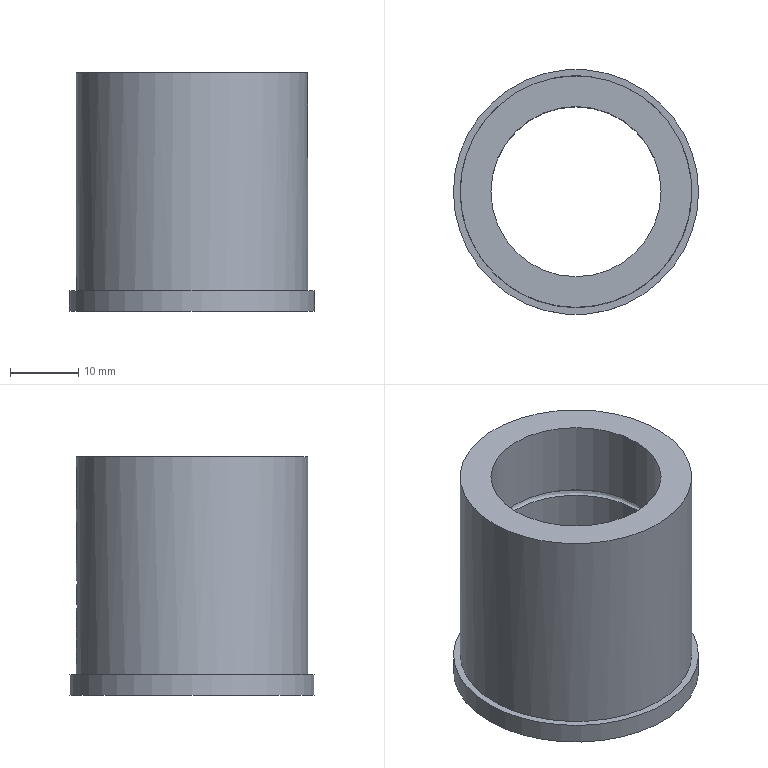Part | NX | features MI_SGBF_0296 2 | 1 solid | 140 faces | box 36 x 36 x 35 mm | volume 14860 mm3 | plane 77 | cylinder 61 | spline 2 | commonest cylinder face diameters 33.8 x9 25 x3 34 x3 1.74 x2 1.838 x2 2.423 x2